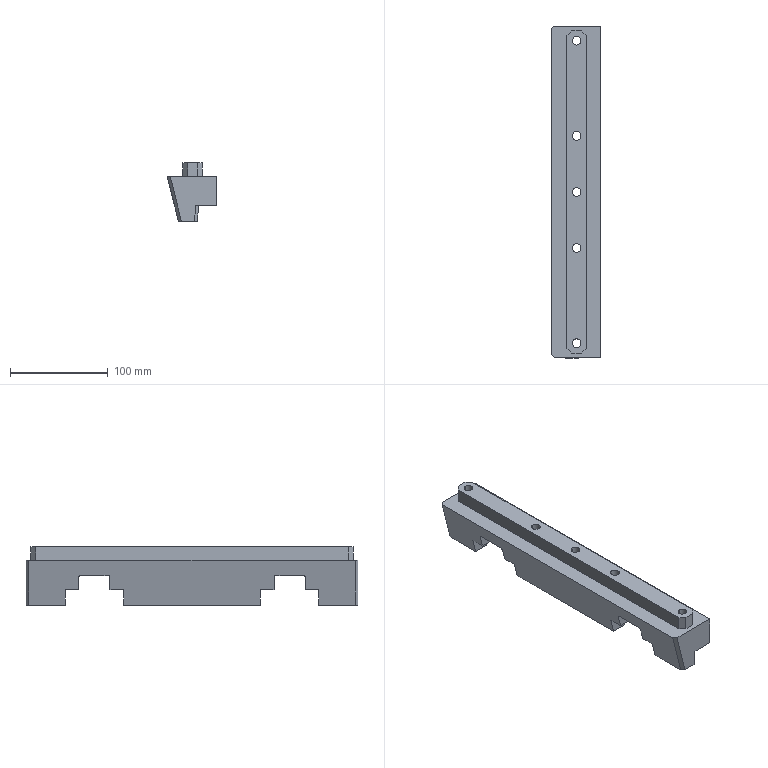Part | Creo | 1 solid | 163 faces | box 50.783 x 340 x 60 mm | volume 576955 mm3 | plane 99 | other 37 | cylinder 27 | commonest cylinder face diameters 9 x10 14 x10 4 x4 11.472 x1 11.957 x1 45.582 x1